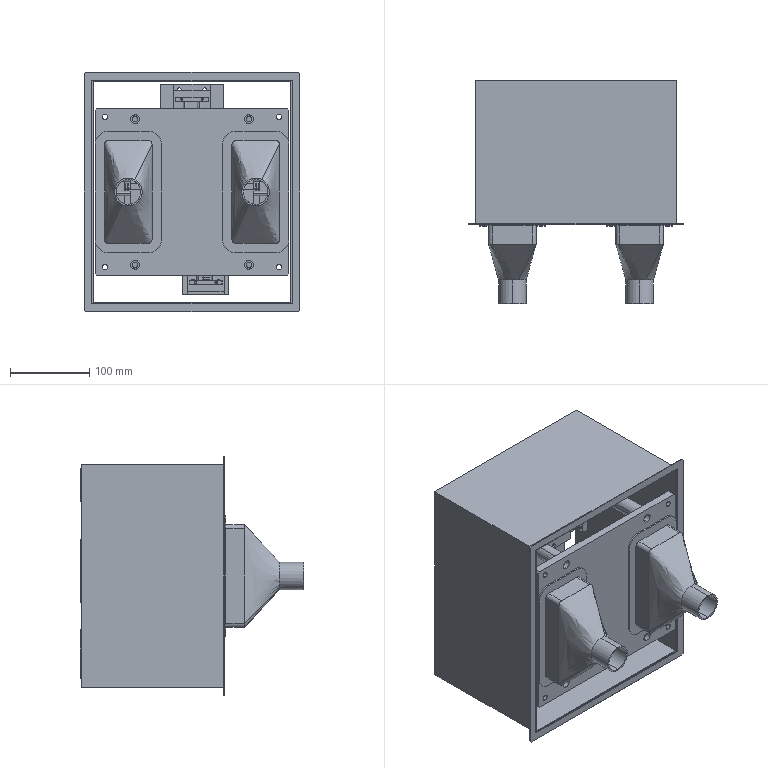Part | SolidWorks | features InContextFeatHolder 4 | 28 solids | 1467 faces | box 273 x 282 x 303 mm | volume 1781179 mm3 | plane 643 | cylinder 546 | cone 268 | spline 10 | commonest cylinder face diameters 0.4 x104 6 x96 10 x40 3.5 x36 2.459 x32 9 x32